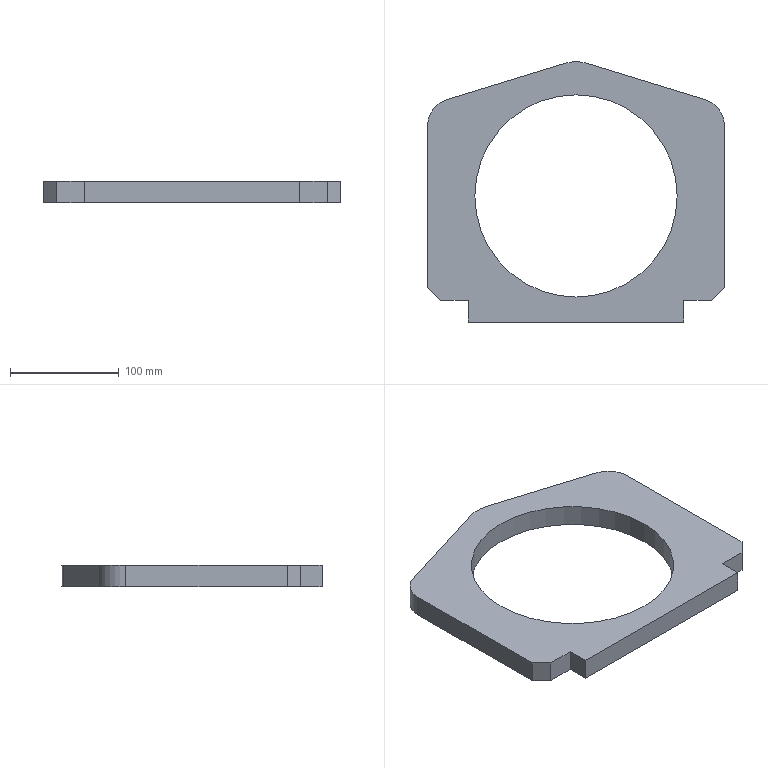Part | SolidWorks | features Extrusion 1 | 1 solid | 18 faces | box 273 x 239.5 x 20 mm | volume 622595 mm3 | plane 13 | cylinder 5 | commonest cylinder face diameters 50 x2 186 x2 70 x1
STEP:
#1=CARTESIAN_POINT('',(-93.,116.,20.));
#2=VERTEX_POINT('',#1);
#3=CARTESIAN_POINT('',(93.,116.,20.));
#4=VERTEX_POINT('',#3);
#5=CARTESIAN_POINT('',(0.,116.,20.));
#6=DIRECTION('',(0.,0.,1.));
#7=DIRECTION('',(1.,0.,0.));
#8=AXIS2_PLACEMENT_3D('',#5,#6,#7);
#9=CIRCLE('',#8,93.);
#10=EDGE_CURVE('',#2,#4,#9,.T.);
#11=ORIENTED_EDGE('',*,*,#10,.T.);
#12=CARTESIAN_POINT('',(93.,116.,0.));
#13=VERTEX_POINT('',#12);
#14=CARTESIAN_POINT('',(93.,116.,20.));
#15=DIRECTION('',(0.,0.,-1.));
#16=VECTOR('',#15,1000.);
#17=LINE('',#14,#16);
#18=EDGE_CURVE('',#4,#13,#17,.T.);
#19=ORIENTED_EDGE('',*,*,#18,.T.);
#20=CARTESIAN_POINT('',(-93.,116.,0.));
#21=VERTEX_POINT('',#20);
#22=CARTESIAN_POINT('',(0.,116.,0.));
#23=DIRECTION('',(0.,0.,1.));
#24=DIRECTION('',(1.,0.,0.));
#25=AXIS2_PLACEMENT_3D('',#22,#23,#24);
#26=CIRCLE('',#25,93.);
#27=EDGE_CURVE('',#21,#13,#26,.T.);
#28=ORIENTED_EDGE('',*,*,#27,.F.);
#29=CARTESIAN_POINT('',(-93.,116.,20.));
#30=DIRECTION('',(0.,0.,-1.));
#31=VECTOR('',#30,1000.);
#32=LINE('',#29,#31);
#33=EDGE_CURVE('',#2,#21,#32,.T.);
#34=ORIENTED_EDGE('',*,*,#33,.F.);
#35=EDGE_LOOP('',(#11,#19,#28,#34));
#36=FACE_OUTER_BOUND('',#35,.T.);
#37=CARTESIAN_POINT('',(0.,116.,20.));
#38=DIRECTION('',(0.,0.,-1.));
#39=DIRECTION('',(-1.,0.,0.));
#40=AXIS2_PLACEMENT_3D('',#37,#38,#39);
#41=CYLINDRICAL_SURFACE('',#40,93.);
#42=ADVANCED_FACE('',(#36),#41,.F.);
#43=CARTESIAN_POINT('',(99.,0.,20.));
#44=VERTEX_POINT('',#43);
#45=CARTESIAN_POINT('',(99.,20.,20.));
#46=VERTEX_POINT('',#45);
#47=CARTESIAN_POINT('',(99.,0.,20.));
#48=DIRECTION('',(0.,1.,0.));
#49=VECTOR('',#48,1000.);
#50=LINE('',#47,#49);
#51=EDGE_CURVE('',#44,#46,#50,.T.);
#52=ORIENTED_EDGE('',*,*,#51,.T.);
#53=CARTESIAN_POINT('',(124.5,20.,20.));
#54=VERTEX_POINT('',#53);
#55=CARTESIAN_POINT('',(99.,20.,20.));
#56=DIRECTION('',(1.,0.,0.));
#57=VECTOR('',#56,1000.);
#58=LINE('',#55,#57);
#59=EDGE_CURVE('',#46,#54,#58,.T.);
#60=ORIENTED_EDGE('',*,*,#59,.T.);
#61=CARTESIAN_POINT('',(136.5,32.,20.));
#62=VERTEX_POINT('',#61);
#63=CARTESIAN_POINT('',(124.5,20.,20.));
#64=DIRECTION('',(0.7071,0.7071,0.));
#65=VECTOR('',#64,1000.);
#66=LINE('',#63,#65);
#67=EDGE_CURVE('',#54,#62,#66,.T.);
#68=ORIENTED_EDGE('',*,*,#67,.T.);
#69=CARTESIAN_POINT('',(136.5,180.6,20.));
#70=VERTEX_POINT('',#69);
#71=CARTESIAN_POINT('',(136.5,32.,20.));
#72=DIRECTION('',(0.,1.,0.));
#73=VECTOR('',#72,1000.);
#74=LINE('',#71,#73);
#75=EDGE_CURVE('',#62,#70,#74,.T.);
#76=ORIENTED_EDGE('',*,*,#75,.T.);
#77=CARTESIAN_POINT('',(118.863,204.491,20.));
#78=VERTEX_POINT('',#77);
#79=CARTESIAN_POINT('',(111.5,180.6,20.));
#80=DIRECTION('',(0.,0.,1.));
#81=DIRECTION('',(1.,0.,0.));
#82=AXIS2_PLACEMENT_3D('',#79,#80,#81);
#83=CIRCLE('',#82,25.);
#84=EDGE_CURVE('',#70,#78,#83,.T.);
#85=ORIENTED_EDGE('',*,*,#84,.T.);
#86=CARTESIAN_POINT('',(10.308,237.948,20.));
#87=VERTEX_POINT('',#86);
#88=CARTESIAN_POINT('',(10.308,237.948,20.));
#89=DIRECTION('',(-0.9556,0.2945,0.));
#90=VECTOR('',#89,1000.);
#91=LINE('',#88,#90);
#92=EDGE_CURVE('',#78,#87,#91,.T.);
#93=ORIENTED_EDGE('',*,*,#92,.T.);
#94=CARTESIAN_POINT('',(-10.308,237.948,20.));
#95=VERTEX_POINT('',#94);
#96=CARTESIAN_POINT('',(0.,204.5,20.));
#97=DIRECTION('',(0.,0.,1.));
#98=DIRECTION('',(1.,0.,0.));
#99=AXIS2_PLACEMENT_3D('',#96,#97,#98);
#100=CIRCLE('',#99,35.);
#101=EDGE_CURVE('',#87,#95,#100,.T.);
#102=ORIENTED_EDGE('',*,*,#101,.T.);
#103=CARTESIAN_POINT('',(-118.863,204.491,20.));
#104=VERTEX_POINT('',#103);
#105=CARTESIAN_POINT('',(-10.308,237.948,20.));
#106=DIRECTION('',(-0.9556,-0.2945,0.));
#107=VECTOR('',#106,1000.);
#108=LINE('',#105,#107);
#109=EDGE_CURVE('',#95,#104,#108,.T.);
#110=ORIENTED_EDGE('',*,*,#109,.T.);
#111=CARTESIAN_POINT('',(-136.5,180.6,20.));
#112=VERTEX_POINT('',#111);
#113=CARTESIAN_POINT('',(-111.5,180.6,20.));
#114=DIRECTION('',(0.,0.,1.));
#115=DIRECTION('',(-1.,0.,0.));
#116=AXIS2_PLACEMENT_3D('',#113,#114,#115);
#117=CIRCLE('',#116,25.);
#118=EDGE_CURVE('',#104,#112,#117,.T.);
#119=ORIENTED_EDGE('',*,*,#118,.T.);
#120=CARTESIAN_POINT('',(-136.5,32.,20.));
#121=VERTEX_POINT('',#120);
#122=CARTESIAN_POINT('',(-136.5,32.,20.));
#123=DIRECTION('',(0.,-1.,0.));
#124=VECTOR('',#123,1000.);
#125=LINE('',#122,#124);
#126=EDGE_CURVE('',#112,#121,#125,.T.);
#127=ORIENTED_EDGE('',*,*,#126,.T.);
#128=CARTESIAN_POINT('',(-124.5,20.,20.));
#129=VERTEX_POINT('',#128);
#130=CARTESIAN_POINT('',(-124.5,20.,20.));
#131=DIRECTION('',(0.7071,-0.7071,0.));
#132=VECTOR('',#131,1000.);
#133=LINE('',#130,#132);
#134=EDGE_CURVE('',#121,#129,#133,.T.);
#135=ORIENTED_EDGE('',*,*,#134,.T.);
#136=CARTESIAN_POINT('',(-99.,20.,20.));
#137=VERTEX_POINT('',#136);
#138=CARTESIAN_POINT('',(-99.,20.,20.));
#139=DIRECTION('',(1.,0.,0.));
#140=VECTOR('',#139,1000.);
#141=LINE('',#138,#140);
#142=EDGE_CURVE('',#129,#137,#141,.T.);
#143=ORIENTED_EDGE('',*,*,#142,.T.);
#144=CARTESIAN_POINT('',(-99.,0.,20.));
#145=VERTEX_POINT('',#144);
#146=CARTESIAN_POINT('',(-99.,0.,20.));
#147=DIRECTION('',(0.,-1.,0.));
#148=VECTOR('',#147,1000.);
#149=LINE('',#146,#148);
#150=EDGE_CURVE('',#137,#145,#149,.T.);
#151=ORIENTED_EDGE('',*,*,#150,.T.);
#152=CARTESIAN_POINT('',(-99.,0.,20.));
#153=DIRECTION('',(1.,0.,0.));
#154=VECTOR('',#153,1000.);
#155=LINE('',#152,#154);
#156=EDGE_CURVE('',#145,#44,#155,.T.);
#157=ORIENTED_EDGE('',*,*,#156,.T.);
#158=EDGE_LOOP('',(#52,#60,#68,#76,#85,#93,#102,#110,#119,#127,#135,#143,#151,#157));
#159=FACE_OUTER_BOUND('',#158,.T.);
#160=ORIENTED_EDGE('',*,*,#10,.F.);
#161=CARTESIAN_POINT('',(0.,116.,20.));
#162=DIRECTION('',(0.,0.,1.));
#163=DIRECTION('',(1.,0.,0.));
#164=AXIS2_PLACEMENT_3D('',#161,#162,#163);
#165=CIRCLE('',#164,93.);
#166=EDGE_CURVE('',#4,#2,#165,.T.);
#167=ORIENTED_EDGE('',*,*,#166,.F.);
#168=EDGE_LOOP('',(#160,#167));
#169=FACE_BOUND('',#168,.T.);
#170=CARTESIAN_POINT('',(111.5,180.6,20.));
#171=DIRECTION('',(0.,0.,1.));
#172=DIRECTION('',(1.,0.,0.));
#173=AXIS2_PLACEMENT_3D('',#170,#171,#172);
#174=PLANE('',#173);
#175=ADVANCED_FACE('',(#159,#169),#174,.T.);
#176=CARTESIAN_POINT('',(99.,0.,0.));
#177=VERTEX_POINT('',#176);
#178=CARTESIAN_POINT('',(99.,20.,0.));
#179=VERTEX_POINT('',#178);
#180=CARTESIAN_POINT('',(99.,0.,0.));
#181=DIRECTION('',(0.,1.,0.));
#182=VECTOR('',#181,1000.);
#183=LINE('',#180,#182);
#184=EDGE_CURVE('',#177,#179,#183,.T.);
#185=ORIENTED_EDGE('',*,*,#184,.F.);
#186=CARTESIAN_POINT('',(-99.,0.,0.));
#187=VERTEX_POINT('',#186);
#188=CARTESIAN_POINT('',(-99.,0.,0.));
#189=DIRECTION('',(1.,0.,0.));
#190=VECTOR('',#189,1000.);
#191=LINE('',#188,#190);
#192=EDGE_CURVE('',#187,#177,#191,.T.);
#193=ORIENTED_EDGE('',*,*,#192,.F.);
#194=CARTESIAN_POINT('',(-99.,20.,0.));
#195=VERTEX_POINT('',#194);
#196=CARTESIAN_POINT('',(-99.,0.,0.));
#197=DIRECTION('',(0.,-1.,0.));
#198=VECTOR('',#197,1000.);
#199=LINE('',#196,#198);
#200=EDGE_CURVE('',#195,#187,#199,.T.);
#201=ORIENTED_EDGE('',*,*,#200,.F.);
#202=CARTESIAN_POINT('',(-124.5,20.,0.));
#203=VERTEX_POINT('',#202);
#204=CARTESIAN_POINT('',(-99.,20.,0.));
#205=DIRECTION('',(1.,0.,0.));
#206=VECTOR('',#205,1000.);
#207=LINE('',#204,#206);
#208=EDGE_CURVE('',#203,#195,#207,.T.);
#209=ORIENTED_EDGE('',*,*,#208,.F.);
#210=CARTESIAN_POINT('',(-136.5,32.,0.));
#211=VERTEX_POINT('',#210);
#212=CARTESIAN_POINT('',(-124.5,20.,0.));
#213=DIRECTION('',(0.7071,-0.7071,0.));
#214=VECTOR('',#213,1000.);
#215=LINE('',#212,#214);
#216=EDGE_CURVE('',#211,#203,#215,.T.);
#217=ORIENTED_EDGE('',*,*,#216,.F.);
#218=CARTESIAN_POINT('',(-136.5,180.6,0.));
#219=VERTEX_POINT('',#218);
#220=CARTESIAN_POINT('',(-136.5,32.,0.));
#221=DIRECTION('',(0.,-1.,0.));
#222=VECTOR('',#221,1000.);
#223=LINE('',#220,#222);
#224=EDGE_CURVE('',#219,#211,#223,.T.);
#225=ORIENTED_EDGE('',*,*,#224,.F.);
#226=CARTESIAN_POINT('',(-118.863,204.491,0.));
#227=VERTEX_POINT('',#226);
#228=CARTESIAN_POINT('',(-111.5,180.6,0.));
#229=DIRECTION('',(0.,0.,1.));
#230=DIRECTION('',(-1.,0.,0.));
#231=AXIS2_PLACEMENT_3D('',#228,#229,#230);
#232=CIRCLE('',#231,25.);
#233=EDGE_CURVE('',#227,#219,#232,.T.);
#234=ORIENTED_EDGE('',*,*,#233,.F.);
#235=CARTESIAN_POINT('',(-10.308,237.948,0.));
#236=VERTEX_POINT('',#235);
#237=CARTESIAN_POINT('',(-10.308,237.948,0.));
#238=DIRECTION('',(-0.9556,-0.2945,0.));
#239=VECTOR('',#238,1000.);
#240=LINE('',#237,#239);
#241=EDGE_CURVE('',#236,#227,#240,.T.);
#242=ORIENTED_EDGE('',*,*,#241,.F.);
#243=CARTESIAN_POINT('',(10.308,237.948,0.));
#244=VERTEX_POINT('',#243);
#245=CARTESIAN_POINT('',(0.,204.5,0.));
#246=DIRECTION('',(0.,0.,1.));
#247=DIRECTION('',(1.,0.,0.));
#248=AXIS2_PLACEMENT_3D('',#245,#246,#247);
#249=CIRCLE('',#248,35.);
#250=EDGE_CURVE('',#244,#236,#249,.T.);
#251=ORIENTED_EDGE('',*,*,#250,.F.);
#252=CARTESIAN_POINT('',(118.863,204.491,0.));
#253=VERTEX_POINT('',#252);
#254=CARTESIAN_POINT('',(10.308,237.948,0.));
#255=DIRECTION('',(-0.9556,0.2945,0.));
#256=VECTOR('',#255,1000.);
#257=LINE('',#254,#256);
#258=EDGE_CURVE('',#253,#244,#257,.T.);
#259=ORIENTED_EDGE('',*,*,#258,.F.);
#260=CARTESIAN_POINT('',(136.5,180.6,0.));
#261=VERTEX_POINT('',#260);
#262=CARTESIAN_POINT('',(111.5,180.6,0.));
#263=DIRECTION('',(0.,0.,1.));
#264=DIRECTION('',(1.,0.,0.));
#265=AXIS2_PLACEMENT_3D('',#262,#263,#264);
#266=CIRCLE('',#265,25.);
#267=EDGE_CURVE('',#261,#253,#266,.T.);
#268=ORIENTED_EDGE('',*,*,#267,.F.);
#269=CARTESIAN_POINT('',(136.5,32.,0.));
#270=VERTEX_POINT('',#269);
#271=CARTESIAN_POINT('',(136.5,32.,0.));
#272=DIRECTION('',(0.,1.,0.));
#273=VECTOR('',#272,1000.);
#274=LINE('',#271,#273);
#275=EDGE_CURVE('',#270,#261,#274,.T.);
#276=ORIENTED_EDGE('',*,*,#275,.F.);
#277=CARTESIAN_POINT('',(124.5,20.,0.));
#278=VERTEX_POINT('',#277);
#279=CARTESIAN_POINT('',(124.5,20.,0.));
#280=DIRECTION('',(0.7071,0.7071,0.));
#281=VECTOR('',#280,1000.);
#282=LINE('',#279,#281);
#283=EDGE_CURVE('',#278,#270,#282,.T.);
#284=ORIENTED_EDGE('',*,*,#283,.F.);
#285=CARTESIAN_POINT('',(99.,20.,0.));
#286=DIRECTION('',(1.,0.,0.));
#287=VECTOR('',#286,1000.);
#288=LINE('',#285,#287);
#289=EDGE_CURVE('',#179,#278,#288,.T.);
#290=ORIENTED_EDGE('',*,*,#289,.F.);
#291=EDGE_LOOP('',(#185,#193,#201,#209,#217,#225,#234,#242,#251,#259,#268,#276,#284,#290));
#292=FACE_OUTER_BOUND('',#291,.T.);
#293=ORIENTED_EDGE('',*,*,#27,.T.);
#294=CARTESIAN_POINT('',(0.,116.,0.));
#295=DIRECTION('',(0.,0.,1.));
#296=DIRECTION('',(1.,0.,0.));
#297=AXIS2_PLACEMENT_3D('',#294,#295,#296);
#298=CIRCLE('',#297,93.);
#299=EDGE_CURVE('',#13,#21,#298,.T.);
#300=ORIENTED_EDGE('',*,*,#299,.T.);
#301=EDGE_LOOP('',(#293,#300));
#302=FACE_BOUND('',#301,.T.);
#303=CARTESIAN_POINT('',(111.5,180.6,0.));
#304=DIRECTION('',(0.,0.,1.));
#305=DIRECTION('',(1.,0.,0.));
#306=AXIS2_PLACEMENT_3D('',#303,#304,#305);
#307=PLANE('',#306);
#308=ADVANCED_FACE('',(#292,#302),#307,.F.);
#309=ORIENTED_EDGE('',*,*,#184,.T.);
#310=CARTESIAN_POINT('',(99.,20.,20.));
#311=DIRECTION('',(0.,0.,-1.));
#312=VECTOR('',#311,1000.);
#313=LINE('',#310,#312);
#314=EDGE_CURVE('',#46,#179,#313,.T.);
#315=ORIENTED_EDGE('',*,*,#314,.F.);
#316=ORIENTED_EDGE('',*,*,#51,.F.);
#317=CARTESIAN_POINT('',(99.,0.,20.));
#318=DIRECTION('',(0.,0.,-1.));
#319=VECTOR('',#318,1000.);
#320=LINE('',#317,#319);
#321=EDGE_CURVE('',#44,#177,#320,.T.);
#322=ORIENTED_EDGE('',*,*,#321,.T.);
#323=EDGE_LOOP('',(#309,#315,#316,#322));
#324=FACE_OUTER_BOUND('',#323,.T.);
#325=CARTESIAN_POINT('',(99.,0.,20.));
#326=DIRECTION('',(-1.,0.,0.));
#327=DIRECTION('',(0.,0.,1.));
#328=AXIS2_PLACEMENT_3D('',#325,#326,#327);
#329=PLANE('',#328);
#330=ADVANCED_FACE('',(#324),#329,.F.);
#331=ORIENTED_EDGE('',*,*,#289,.T.);
#332=CARTESIAN_POINT('',(124.5,20.,20.));
#333=DIRECTION('',(0.,0.,-1.));
#334=VECTOR('',#333,1000.);
#335=LINE('',#332,#334);
#336=EDGE_CURVE('',#54,#278,#335,.T.);
#337=ORIENTED_EDGE('',*,*,#336,.F.);
#338=ORIENTED_EDGE('',*,*,#59,.F.);
#339=ORIENTED_EDGE('',*,*,#314,.T.);
#340=EDGE_LOOP('',(#331,#337,#338,#339));
#341=FACE_OUTER_BOUND('',#340,.T.);
#342=CARTESIAN_POINT('',(99.,20.,20.));
#343=DIRECTION('',(0.,1.,0.));
#344=DIRECTION('',(0.,0.,1.));
#345=AXIS2_PLACEMENT_3D('',#342,#343,#344);
#346=PLANE('',#345);
#347=ADVANCED_FACE('',(#341),#346,.F.);
#348=ORIENTED_EDGE('',*,*,#283,.T.);
#349=CARTESIAN_POINT('',(136.5,32.,20.));
#350=DIRECTION('',(0.,0.,-1.));
#351=VECTOR('',#350,1000.);
#352=LINE('',#349,#351);
#353=EDGE_CURVE('',#62,#270,#352,.T.);
#354=ORIENTED_EDGE('',*,*,#353,.F.);
#355=ORIENTED_EDGE('',*,*,#67,.F.);
#356=ORIENTED_EDGE('',*,*,#336,.T.);
#357=EDGE_LOOP('',(#348,#354,#355,#356));
#358=FACE_OUTER_BOUND('',#357,.T.);
#359=CARTESIAN_POINT('',(124.5,20.,20.));
#360=DIRECTION('',(-0.7071,0.7071,0.));
#361=DIRECTION('',(-0.7071,-0.7071,0.));
#362=AXIS2_PLACEMENT_3D('',#359,#360,#361);
#363=PLANE('',#362);
#364=ADVANCED_FACE('',(#358),#363,.F.);
#365=ORIENTED_EDGE('',*,*,#275,.T.);
#366=CARTESIAN_POINT('',(136.5,180.6,20.));
#367=DIRECTION('',(0.,0.,-1.));
#368=VECTOR('',#367,1000.);
#369=LINE('',#366,#368);
#370=EDGE_CURVE('',#70,#261,#369,.T.);
#371=ORIENTED_EDGE('',*,*,#370,.F.);
#372=ORIENTED_EDGE('',*,*,#75,.F.);
#373=ORIENTED_EDGE('',*,*,#353,.T.);
#374=EDGE_LOOP('',(#365,#371,#372,#373));
#375=FACE_OUTER_BOUND('',#374,.T.);
#376=CARTESIAN_POINT('',(136.5,32.,20.));
#377=DIRECTION('',(-1.,0.,0.));
#378=DIRECTION('',(0.,0.,1.));
#379=AXIS2_PLACEMENT_3D('',#376,#377,#378);
#380=PLANE('',#379);
#381=ADVANCED_FACE('',(#375),#380,.F.);
#382=ORIENTED_EDGE('',*,*,#267,.T.);
#383=CARTESIAN_POINT('',(118.863,204.491,20.));
#384=DIRECTION('',(0.,0.,-1.));
#385=VECTOR('',#384,1000.);
#386=LINE('',#383,#385);
#387=EDGE_CURVE('',#78,#253,#386,.T.);
#388=ORIENTED_EDGE('',*,*,#387,.F.);
#389=ORIENTED_EDGE('',*,*,#84,.F.);
#390=ORIENTED_EDGE('',*,*,#370,.T.);
#391=EDGE_LOOP('',(#382,#388,#389,#390));
#392=FACE_OUTER_BOUND('',#391,.T.);
#393=CARTESIAN_POINT('',(111.5,180.6,20.));
#394=DIRECTION('',(0.,0.,-1.));
#395=DIRECTION('',(-1.,0.,0.));
#396=AXIS2_PLACEMENT_3D('',#393,#394,#395);
#397=CYLINDRICAL_SURFACE('',#396,25.);
#398=ADVANCED_FACE('',(#392),#397,.T.);
#399=ORIENTED_EDGE('',*,*,#258,.T.);
#400=CARTESIAN_POINT('',(10.308,237.948,20.));
#401=DIRECTION('',(0.,0.,-1.));
#402=VECTOR('',#401,1000.);
#403=LINE('',#400,#402);
#404=EDGE_CURVE('',#87,#244,#403,.T.);
#405=ORIENTED_EDGE('',*,*,#404,.F.);
#406=ORIENTED_EDGE('',*,*,#92,.F.);
#407=ORIENTED_EDGE('',*,*,#387,.T.);
#408=EDGE_LOOP('',(#399,#405,#406,#407));
#409=FACE_OUTER_BOUND('',#408,.T.);
#410=CARTESIAN_POINT('',(10.308,237.948,20.));
#411=DIRECTION('',(-0.2945,-0.9556,0.));
#412=DIRECTION('',(0.9556,-0.2945,0.));
#413=AXIS2_PLACEMENT_3D('',#410,#411,#412);
#414=PLANE('',#413);
#415=ADVANCED_FACE('',(#409),#414,.F.);
#416=ORIENTED_EDGE('',*,*,#250,.T.);
#417=CARTESIAN_POINT('',(-10.308,237.948,20.));
#418=DIRECTION('',(0.,0.,-1.));
#419=VECTOR('',#418,1000.);
#420=LINE('',#417,#419);
#421=EDGE_CURVE('',#95,#236,#420,.T.);
#422=ORIENTED_EDGE('',*,*,#421,.F.);
#423=ORIENTED_EDGE('',*,*,#101,.F.);
#424=ORIENTED_EDGE('',*,*,#404,.T.);
#425=EDGE_LOOP('',(#416,#422,#423,#424));
#426=FACE_OUTER_BOUND('',#425,.T.);
#427=CARTESIAN_POINT('',(0.,204.5,20.));
#428=DIRECTION('',(0.,0.,-1.));
#429=DIRECTION('',(-1.,0.,0.));
#430=AXIS2_PLACEMENT_3D('',#427,#428,#429);
#431=CYLINDRICAL_SURFACE('',#430,35.);
#432=ADVANCED_FACE('',(#426),#431,.T.);
#433=ORIENTED_EDGE('',*,*,#241,.T.);
#434=CARTESIAN_POINT('',(-118.863,204.491,20.));
#435=DIRECTION('',(0.,0.,-1.));
#436=VECTOR('',#435,1000.);
#437=LINE('',#434,#436);
#438=EDGE_CURVE('',#104,#227,#437,.T.);
#439=ORIENTED_EDGE('',*,*,#438,.F.);
#440=ORIENTED_EDGE('',*,*,#109,.F.);
#441=ORIENTED_EDGE('',*,*,#421,.T.);
#442=EDGE_LOOP('',(#433,#439,#440,#441));
#443=FACE_OUTER_BOUND('',#442,.T.);
#444=CARTESIAN_POINT('',(-10.308,237.948,20.));
#445=DIRECTION('',(0.2945,-0.9556,0.));
#446=DIRECTION('',(0.9556,0.2945,0.));
#447=AXIS2_PLACEMENT_3D('',#444,#445,#446);
#448=PLANE('',#447);
#449=ADVANCED_FACE('',(#443),#448,.F.);
#450=ORIENTED_EDGE('',*,*,#233,.T.);
#451=CARTESIAN_POINT('',(-136.5,180.6,20.));
#452=DIRECTION('',(0.,0.,-1.));
#453=VECTOR('',#452,1000.);
#454=LINE('',#451,#453);
#455=EDGE_CURVE('',#112,#219,#454,.T.);
#456=ORIENTED_EDGE('',*,*,#455,.F.);
#457=ORIENTED_EDGE('',*,*,#118,.F.);
#458=ORIENTED_EDGE('',*,*,#438,.T.);
#459=EDGE_LOOP('',(#450,#456,#457,#458));
#460=FACE_OUTER_BOUND('',#459,.T.);
#461=CARTESIAN_POINT('',(-111.5,180.6,20.));
#462=DIRECTION('',(0.,0.,-1.));
#463=DIRECTION('',(-1.,0.,0.));
#464=AXIS2_PLACEMENT_3D('',#461,#462,#463);
#465=CYLINDRICAL_SURFACE('',#464,25.);
#466=ADVANCED_FACE('',(#460),#465,.T.);
#467=ORIENTED_EDGE('',*,*,#224,.T.);
#468=CARTESIAN_POINT('',(-136.5,32.,20.));
#469=DIRECTION('',(0.,0.,-1.));
#470=VECTOR('',#469,1000.);
#471=LINE('',#468,#470);
#472=EDGE_CURVE('',#121,#211,#471,.T.);
#473=ORIENTED_EDGE('',*,*,#472,.F.);
#474=ORIENTED_EDGE('',*,*,#126,.F.);
#475=ORIENTED_EDGE('',*,*,#455,.T.);
#476=EDGE_LOOP('',(#467,#473,#474,#475));
#477=FACE_OUTER_BOUND('',#476,.T.);
#478=CARTESIAN_POINT('',(-136.5,32.,20.));
#479=DIRECTION('',(1.,0.,0.));
#480=DIRECTION('',(0.,0.,-1.));
#481=AXIS2_PLACEMENT_3D('',#478,#479,#480);
#482=PLANE('',#481);
#483=ADVANCED_FACE('',(#477),#482,.F.);
#484=ORIENTED_EDGE('',*,*,#216,.T.);
#485=CARTESIAN_POINT('',(-124.5,20.,20.));
#486=DIRECTION('',(0.,0.,-1.));
#487=VECTOR('',#486,1000.);
#488=LINE('',#485,#487);
#489=EDGE_CURVE('',#129,#203,#488,.T.);
#490=ORIENTED_EDGE('',*,*,#489,.F.);
#491=ORIENTED_EDGE('',*,*,#134,.F.);
#492=ORIENTED_EDGE('',*,*,#472,.T.);
#493=EDGE_LOOP('',(#484,#490,#491,#492));
#494=FACE_OUTER_BOUND('',#493,.T.);
#495=CARTESIAN_POINT('',(-124.5,20.,20.));
#496=DIRECTION('',(0.7071,0.7071,0.));
#497=DIRECTION('',(-0.7071,0.7071,0.));
#498=AXIS2_PLACEMENT_3D('',#495,#496,#497);
#499=PLANE('',#498);
#500=ADVANCED_FACE('',(#494),#499,.F.);
#501=ORIENTED_EDGE('',*,*,#208,.T.);
#502=CARTESIAN_POINT('',(-99.,20.,20.));
#503=DIRECTION('',(0.,0.,-1.));
#504=VECTOR('',#503,1000.);
#505=LINE('',#502,#504);
#506=EDGE_CURVE('',#137,#195,#505,.T.);
#507=ORIENTED_EDGE('',*,*,#506,.F.);
#508=ORIENTED_EDGE('',*,*,#142,.F.);
#509=ORIENTED_EDGE('',*,*,#489,.T.);
#510=EDGE_LOOP('',(#501,#507,#508,#509));
#511=FACE_OUTER_BOUND('',#510,.T.);
#512=CARTESIAN_POINT('',(-99.,20.,20.));
#513=DIRECTION('',(0.,1.,0.));
#514=DIRECTION('',(0.,0.,1.));
#515=AXIS2_PLACEMENT_3D('',#512,#513,#514);
#516=PLANE('',#515);
#517=ADVANCED_FACE('',(#511),#516,.F.);
#518=ORIENTED_EDGE('',*,*,#200,.T.);
#519=CARTESIAN_POINT('',(-99.,0.,20.));
#520=DIRECTION('',(0.,0.,-1.));
#521=VECTOR('',#520,1000.);
#522=LINE('',#519,#521);
#523=EDGE_CURVE('',#145,#187,#522,.T.);
#524=ORIENTED_EDGE('',*,*,#523,.F.);
#525=ORIENTED_EDGE('',*,*,#150,.F.);
#526=ORIENTED_EDGE('',*,*,#506,.T.);
#527=EDGE_LOOP('',(#518,#524,#525,#526));
#528=FACE_OUTER_BOUND('',#527,.T.);
#529=CARTESIAN_POINT('',(-99.,0.,20.));
#530=DIRECTION('',(1.,0.,0.));
#531=DIRECTION('',(0.,0.,-1.));
#532=AXIS2_PLACEMENT_3D('',#529,#530,#531);
#533=PLANE('',#532);
#534=ADVANCED_FACE('',(#528),#533,.F.);
#535=ORIENTED_EDGE('',*,*,#192,.T.);
#536=ORIENTED_EDGE('',*,*,#321,.F.);
#537=ORIENTED_EDGE('',*,*,#156,.F.);
#538=ORIENTED_EDGE('',*,*,#523,.T.);
#539=EDGE_LOOP('',(#535,#536,#537,#538));
#540=FACE_OUTER_BOUND('',#539,.T.);
#541=CARTESIAN_POINT('',(-99.,0.,20.));
#542=DIRECTION('',(0.,1.,0.));
#543=DIRECTION('',(0.,0.,1.));
#544=AXIS2_PLACEMENT_3D('',#541,#542,#543);
#545=PLANE('',#544);
#546=ADVANCED_FACE('',(#540),#545,.F.);
#547=ORIENTED_EDGE('',*,*,#18,.F.);
#548=ORIENTED_EDGE('',*,*,#166,.T.);
#549=ORIENTED_EDGE('',*,*,#33,.T.);
#550=ORIENTED_EDGE('',*,*,#299,.F.);
#551=EDGE_LOOP('',(#547,#548,#549,#550));
#552=FACE_OUTER_BOUND('',#551,.T.);
#553=CARTESIAN_POINT('',(0.,116.,20.));
#554=DIRECTION('',(0.,0.,-1.));
#555=DIRECTION('',(-1.,0.,0.));
#556=AXIS2_PLACEMENT_3D('',#553,#554,#555);
#557=CYLINDRICAL_SURFACE('',#556,93.);
#558=ADVANCED_FACE('',(#552),#557,.F.);
#559=CLOSED_SHELL('',(#42,#175,#308,#330,#347,#364,#381,#398,#415,#432,#449,#466,#483,#500,#517,#534,#546,#558));
#560=MANIFOLD_SOLID_BREP('',#559);
#561=CARTESIAN_POINT('',(0.,0.,0.));
#562=DIRECTION('',(0.,0.,1.));
#563=DIRECTION('',(1.,0.,0.));
#564=AXIS2_PLACEMENT_3D('',#561,#562,#563);
#565=(LENGTH_UNIT()NAMED_UNIT(*)SI_UNIT(.MILLI.,.METRE.));
#566=UNCERTAINTY_MEASURE_WITH_UNIT(LENGTH_MEASURE(0.00001),#565,'','');
#567=(NAMED_UNIT(*)PLANE_ANGLE_UNIT()SI_UNIT($,.RADIAN.));
#568=(NAMED_UNIT(*)SI_UNIT($,.STERADIAN.)SOLID_ANGLE_UNIT());
#569=(GEOMETRIC_REPRESENTATION_CONTEXT(3)GLOBAL_UNCERTAINTY_ASSIGNED_CONTEXT((#566))GLOBAL_UNIT_ASSIGNED_CONTEXT((#565,#567,#568))REPRESENTATION_CONTEXT('',''));
#570=ADVANCED_BREP_SHAPE_REPRESENTATION('',(#560,#564),#569);